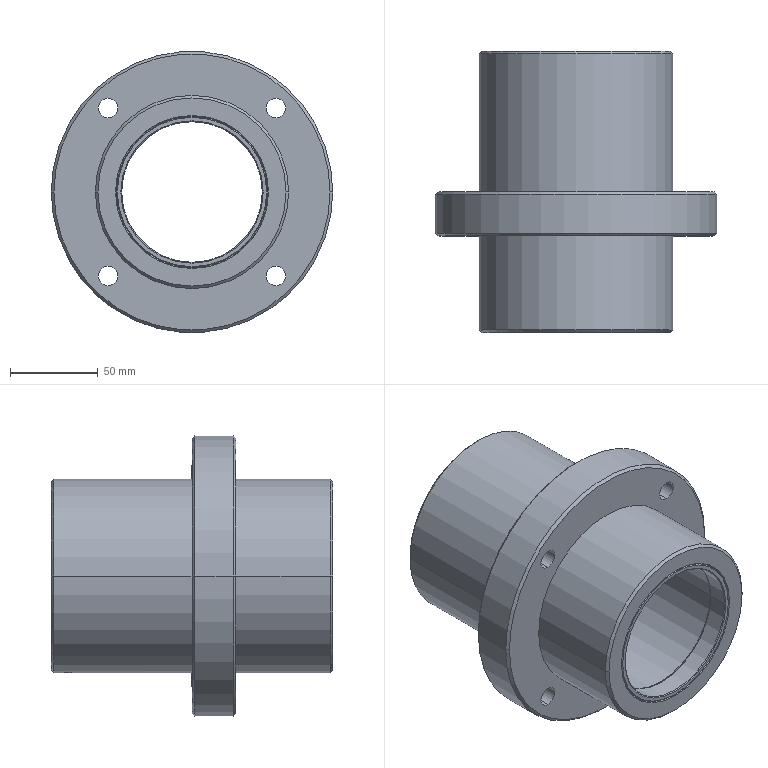Part | SolidWorks | features BaseBody 5 | 5 solids | 122 faces | box 160 x 160 x 160 mm | volume 955059 mm3 | cylinder 58 | cone 40 | plane 24 | commonest cylinder face diameters 11 x8 18 x8 80 x8 85 x8 86 x8 92 x8